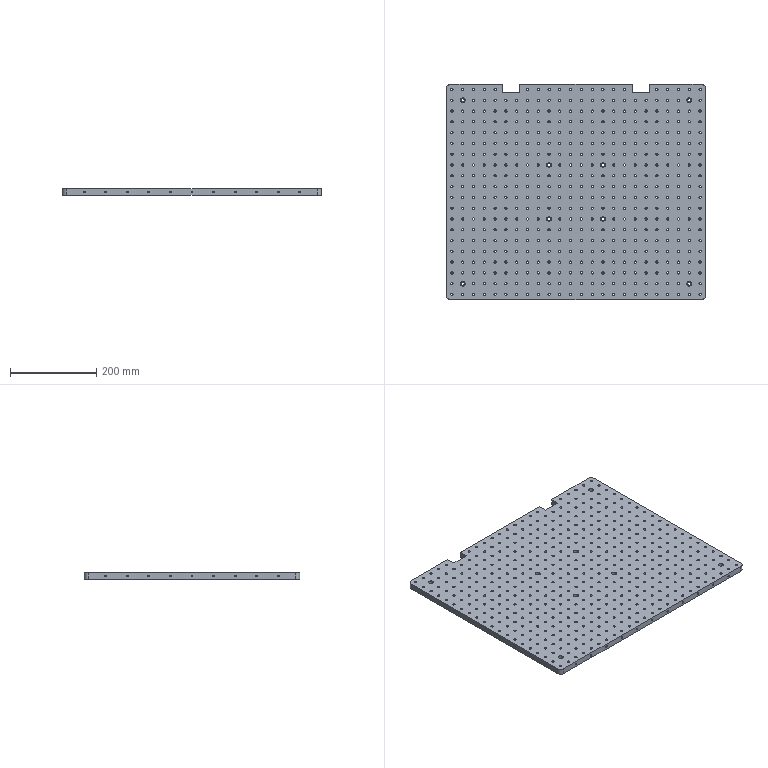Part | SolidWorks | features BaseBody 1 | 1 solid | 1108 faces | box 600 x 500 x 14 mm | volume 4024058 mm3 | cylinder 1048 | plane 60 | commonest cylinder face diameters 5.2 x936 4.2 x76 7 x16 11 x16 20 x4